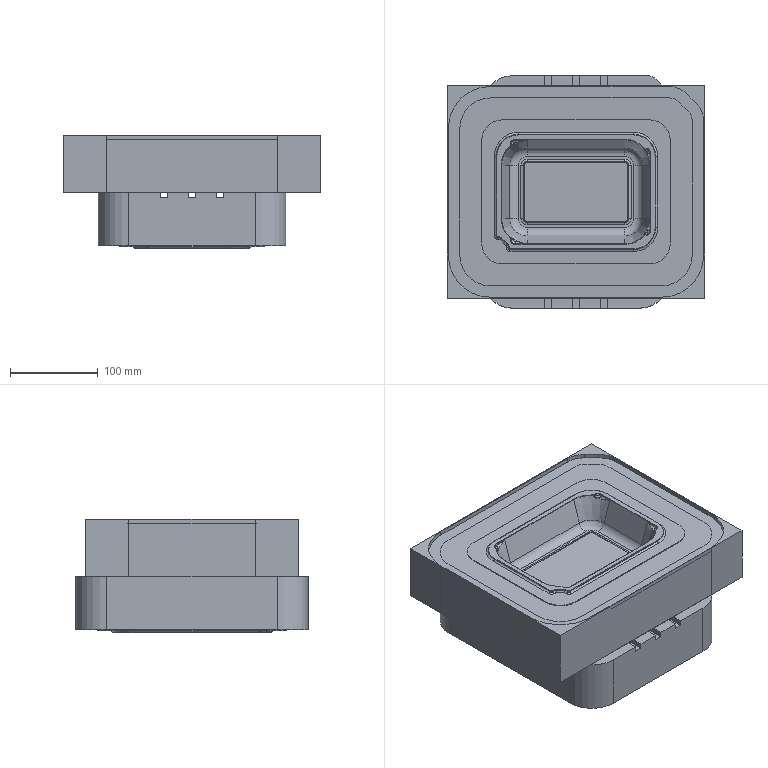NC program | NX | posted with a generic post | part box 293.342 x 265.342 x 129.5 mm
Lines 52945 to 52990 of 68427:
(DRILLING , TOOL : V2.0)
N105870 M6
N105872 G53
N105874 G17 G0 G90 X-38.55 Y70.961 S2000 M3 M8
N105876 G43 Z215.5 H0
N105878 G94 G81 G98 Z59.662 F150. R64.662
N105880 X0.
N105882 X38.549
N105884 X76.842 Y68.887
N105886 X96.371 Y38.549
N105888 Y0.
N105890 Y-38.549
N105892 X76.842 Y-68.887
N105894 X38.549 Y-70.961
N105896 X0.
N105898 X-38.55
N105900 X-76.842 Y-68.888
N105902 X-96.371 Y-38.55
N105904 Y-0.001
N105906 Y38.549
N105908 X-76.842 Y68.887
N105910 X-59.726 Y38.108 Z26.464 R31.464
N105912 X-40. Y32. Z27.959 R32.959
N105914 X-19.961 Y39.093 Z26.464 R31.464
N105916 X0. Y32. Z27.959 R32.959
N105918 X19.961 Y39.093 Z26.464 R31.464
N105920 X40. Y32. Z27.959 R32.959
N105922 X59.726 Y38.108 Z26.464 R31.464
N105924 X64.504 Y0.
N105926 X40.171 Z27.959 R32.959
N105928 X-0.001
N105930 X-40.001
N105932 X-64.504 Z26.464 R31.464
N105934 X-59.726 Y-38.108
N105936 X-40.001 Y-32. Z27.959 R32.959
N105938 X-19.961 Y-39.093 Z26.464 R31.464
N105940 X-0.001 Y-32. Z27.959 R32.959
N105942 X19.961 Y-39.093 Z26.464 R31.464
N105944 X39.999 Y-32. Z27.959 R32.959
N105946 X59.726 Y-38.108 Z26.464 R31.464
N105948 G80
N105950 G0 X59.726 Y-38.108 Z215.5
N105952 M9
N105954 M5